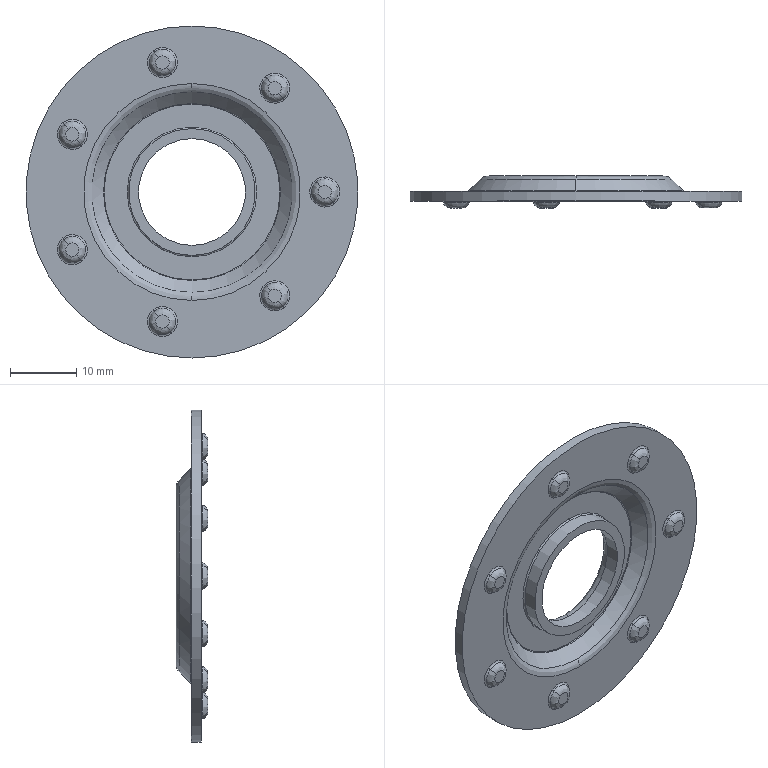Part | STEP file | PRODUTO_ARRUELA | 1 solid | 72 faces | box 50 x 4.8 x 50 mm | volume 2970 mm3 | other 26 | plane 19 | spline 14 | cylinder 10 | cone 3 | commonest cylinder face diameters 2 x7 16.1 x1 19.1 x1 50 x1